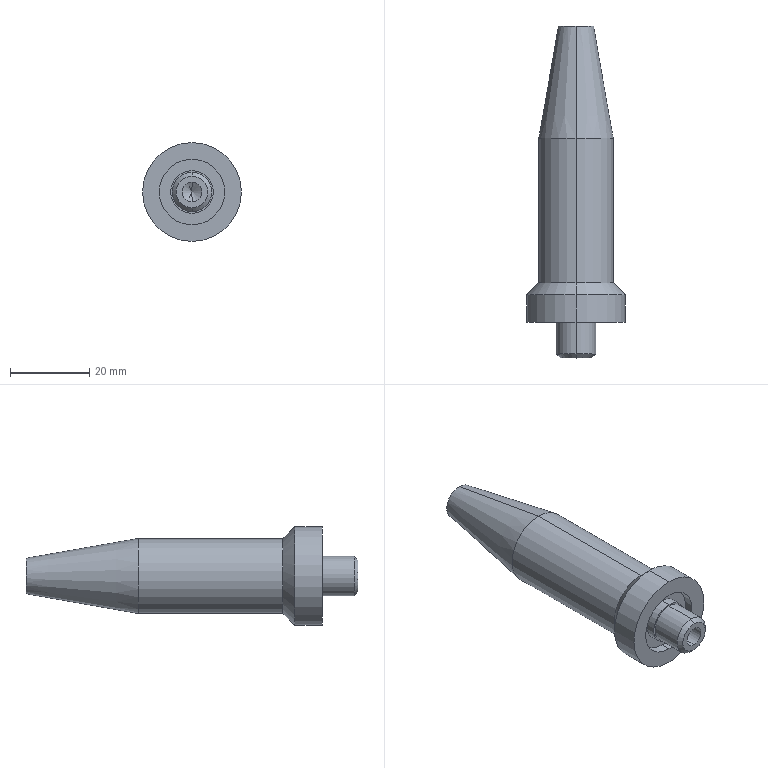Part | STEP file | PN_0062 | 1 solid | 25 faces | box 25 x 84 x 25 mm | volume 19612 mm3 | cylinder 12 | cone 8 | plane 5 | commonest cylinder face diameters 5 x2 10 x2 10.8 x2 16.6 x2 19 x2 25 x2
STEP:
#1=CARTESIAN_POINT('',(0.,0.,0.));
#2=DIRECTION('',(0.,0.,1.));
#3=DIRECTION('',(1.,0.,0.));
#4=AXIS2_PLACEMENT_3D('',#1,#2,#3);
#5=CARTESIAN_POINT('',(0.,75.,4.5));
#6=VERTEX_POINT('',#5);
#7=CARTESIAN_POINT('',(0.,75.,-4.5));
#8=VERTEX_POINT('',#7);
#9=CARTESIAN_POINT('',(0.,75.,0.));
#10=DIRECTION('',(0.,1.,0.));
#11=DIRECTION('',(0.,0.,1.));
#12=AXIS2_PLACEMENT_3D('',#9,#10,#11);
#13=CIRCLE('',#12,4.5);
#14=CARTESIAN_POINT('',(0.,75.,0.));
#15=DIRECTION('',(0.,-1.,0.));
#16=DIRECTION('',(0.,0.,-1.));
#17=AXIS2_PLACEMENT_3D('',#14,#15,#16);
#18=CONICAL_SURFACE('',#17,4.5,0.1745);
#19=CARTESIAN_POINT('',(3.142,0.));
#20=DIRECTION('',(-1.,0.));
#21=VECTOR('',#20,1.);
#22=LINE('',#19,#21);
#23=(GEOMETRIC_REPRESENTATION_CONTEXT(2)PARAMETRIC_REPRESENTATION_CONTEXT()REPRESENTATION_CONTEXT('',''));
#24=DEFINITIONAL_REPRESENTATION('',(#22),#23);
#25=PCURVE('',#18,#24);
#26=CARTESIAN_POINT('',(0.,75.,0.));
#27=DIRECTION('',(0.,1.,0.));
#28=DIRECTION('',(0.,0.,1.));
#29=AXIS2_PLACEMENT_3D('',#26,#27,#28);
#30=PLANE('',#29);
#31=CARTESIAN_POINT('',(0.,0.));
#32=DIRECTION('',(1.,0.));
#33=AXIS2_PLACEMENT_2D('',#31,#32);
#34=CIRCLE('',#33,4.5);
#35=(GEOMETRIC_REPRESENTATION_CONTEXT(2)PARAMETRIC_REPRESENTATION_CONTEXT()REPRESENTATION_CONTEXT('',''));
#36=DEFINITIONAL_REPRESENTATION('',(#34),#35);
#37=PCURVE('',#30,#36);
#38=SURFACE_CURVE('',#13,(#25,#37),.PCURVE_S1.);
#39=EDGE_CURVE('',#6,#8,#38,.T.);
#40=ORIENTED_EDGE('',*,*,#39,.F.);
#41=CARTESIAN_POINT('',(0.,46.644,9.5));
#42=VERTEX_POINT('',#41);
#43=CARTESIAN_POINT('',(0.,75.,4.5));
#44=DIRECTION('',(0.,-0.9848,0.1736));
#45=VECTOR('',#44,1.);
#46=LINE('',#43,#45);
#47=CARTESIAN_POINT('',(3.142,0.));
#48=DIRECTION('',(0.,1.));
#49=VECTOR('',#48,1.);
#50=LINE('',#47,#49);
#51=(GEOMETRIC_REPRESENTATION_CONTEXT(2)PARAMETRIC_REPRESENTATION_CONTEXT()REPRESENTATION_CONTEXT('',''));
#52=DEFINITIONAL_REPRESENTATION('',(#50),#51);
#53=PCURVE('',#18,#52);
#54=CARTESIAN_POINT('',(0.,75.,0.));
#55=DIRECTION('',(0.,-1.,0.));
#56=DIRECTION('',(0.,0.,-1.));
#57=AXIS2_PLACEMENT_3D('',#54,#55,#56);
#58=CONICAL_SURFACE('',#57,4.5,0.1745);
#59=CARTESIAN_POINT('',(3.142,0.));
#60=DIRECTION('',(0.,1.));
#61=VECTOR('',#60,1.);
#62=LINE('',#59,#61);
#63=(GEOMETRIC_REPRESENTATION_CONTEXT(2)PARAMETRIC_REPRESENTATION_CONTEXT()REPRESENTATION_CONTEXT('',''));
#64=DEFINITIONAL_REPRESENTATION('',(#62),#63);
#65=PCURVE('',#58,#64);
#66=SURFACE_CURVE('',#46,(#53,#65),.PCURVE_S1.);
#67=EDGE_CURVE('',#6,#42,#66,.T.);
#68=ORIENTED_EDGE('',*,*,#67,.T.);
#69=CARTESIAN_POINT('',(0.,46.644,-9.5));
#70=VERTEX_POINT('',#69);
#71=CARTESIAN_POINT('',(0.,46.644,0.));
#72=DIRECTION('',(0.,-1.,0.));
#73=DIRECTION('',(0.,0.,1.));
#74=AXIS2_PLACEMENT_3D('',#71,#72,#73);
#75=CIRCLE('',#74,9.5);
#76=CARTESIAN_POINT('',(-3.142,28.356));
#77=DIRECTION('',(1.,0.));
#78=VECTOR('',#77,1.);
#79=LINE('',#76,#78);
#80=(GEOMETRIC_REPRESENTATION_CONTEXT(2)PARAMETRIC_REPRESENTATION_CONTEXT()REPRESENTATION_CONTEXT('',''));
#81=DEFINITIONAL_REPRESENTATION('',(#79),#80);
#82=PCURVE('',#18,#81);
#83=CARTESIAN_POINT('',(0.,75.,0.));
#84=DIRECTION('',(0.,-1.,0.));
#85=DIRECTION('',(0.,0.,-1.));
#86=AXIS2_PLACEMENT_3D('',#83,#84,#85);
#87=CYLINDRICAL_SURFACE('',#86,9.5);
#88=CARTESIAN_POINT('',(-3.142,28.356));
#89=DIRECTION('',(1.,0.));
#90=VECTOR('',#89,1.);
#91=LINE('',#88,#90);
#92=(GEOMETRIC_REPRESENTATION_CONTEXT(2)PARAMETRIC_REPRESENTATION_CONTEXT()REPRESENTATION_CONTEXT('',''));
#93=DEFINITIONAL_REPRESENTATION('',(#91),#92);
#94=PCURVE('',#87,#93);
#95=SURFACE_CURVE('',#75,(#82,#94),.PCURVE_S1.);
#96=EDGE_CURVE('',#70,#42,#95,.T.);
#97=ORIENTED_EDGE('',*,*,#96,.F.);
#98=CARTESIAN_POINT('',(0.,75.,-4.5));
#99=DIRECTION('',(0.,-0.9848,-0.1736));
#100=VECTOR('',#99,1.);
#101=LINE('',#98,#100);
#102=CARTESIAN_POINT('',(0.,0.));
#103=DIRECTION('',(0.,1.));
#104=VECTOR('',#103,1.);
#105=LINE('',#102,#104);
#106=(GEOMETRIC_REPRESENTATION_CONTEXT(2)PARAMETRIC_REPRESENTATION_CONTEXT()REPRESENTATION_CONTEXT('',''));
#107=DEFINITIONAL_REPRESENTATION('',(#105),#106);
#108=PCURVE('',#18,#107);
#109=CARTESIAN_POINT('',(6.283,0.));
#110=DIRECTION('',(0.,1.));
#111=VECTOR('',#110,1.);
#112=LINE('',#109,#111);
#113=(GEOMETRIC_REPRESENTATION_CONTEXT(2)PARAMETRIC_REPRESENTATION_CONTEXT()REPRESENTATION_CONTEXT('',''));
#114=DEFINITIONAL_REPRESENTATION('',(#112),#113);
#115=PCURVE('',#58,#114);
#116=SURFACE_CURVE('',#101,(#108,#115),.PCURVE_S1.);
#117=EDGE_CURVE('',#8,#70,#116,.T.);
#118=ORIENTED_EDGE('',*,*,#117,.F.);
#119=EDGE_LOOP('',(#40,#68,#97,#118));
#120=FACE_BOUND('',#119,.T.);
#121=ADVANCED_FACE('',(#120),#18,.T.);
#122=CARTESIAN_POINT('',(0.,6.,-2.5));
#123=VERTEX_POINT('',#122);
#124=CARTESIAN_POINT('',(0.,-9.,-2.5));
#125=VERTEX_POINT('',#124);
#126=CARTESIAN_POINT('',(0.,-9.,-2.5));
#127=DIRECTION('',(0.,-1.,0.));
#128=VECTOR('',#127,1.);
#129=LINE('',#126,#128);
#130=CARTESIAN_POINT('',(0.,-9.,0.));
#131=DIRECTION('',(0.,-1.,0.));
#132=DIRECTION('',(0.,0.,-1.));
#133=AXIS2_PLACEMENT_3D('',#130,#131,#132);
#134=CYLINDRICAL_SURFACE('',#133,2.5);
#135=CARTESIAN_POINT('',(6.283,0.));
#136=DIRECTION('',(0.,1.));
#137=VECTOR('',#136,1.);
#138=LINE('',#135,#137);
#139=(GEOMETRIC_REPRESENTATION_CONTEXT(2)PARAMETRIC_REPRESENTATION_CONTEXT()REPRESENTATION_CONTEXT('',''));
#140=DEFINITIONAL_REPRESENTATION('',(#138),#139);
#141=PCURVE('',#134,#140);
#142=CARTESIAN_POINT('',(0.,-9.,0.));
#143=DIRECTION('',(0.,-1.,0.));
#144=DIRECTION('',(0.,0.,-1.));
#145=AXIS2_PLACEMENT_3D('',#142,#143,#144);
#146=CYLINDRICAL_SURFACE('',#145,2.5);
#147=CARTESIAN_POINT('',(0.,0.));
#148=DIRECTION('',(0.,1.));
#149=VECTOR('',#148,1.);
#150=LINE('',#147,#149);
#151=(GEOMETRIC_REPRESENTATION_CONTEXT(2)PARAMETRIC_REPRESENTATION_CONTEXT()REPRESENTATION_CONTEXT('',''));
#152=DEFINITIONAL_REPRESENTATION('',(#150),#151);
#153=PCURVE('',#146,#152);
#154=SURFACE_CURVE('',#129,(#141,#153),.PCURVE_S1.);
#155=EDGE_CURVE('',#123,#125,#154,.T.);
#156=ORIENTED_EDGE('',*,*,#155,.T.);
#157=CARTESIAN_POINT('',(0.,-9.,2.5));
#158=VERTEX_POINT('',#157);
#159=CARTESIAN_POINT('',(0.,-9.,0.));
#160=DIRECTION('',(0.,-1.,0.));
#161=DIRECTION('',(0.,0.,-1.));
#162=AXIS2_PLACEMENT_3D('',#159,#160,#161);
#163=CIRCLE('',#162,2.5);
#164=CARTESIAN_POINT('',(0.,0.));
#165=DIRECTION('',(1.,0.));
#166=VECTOR('',#165,1.);
#167=LINE('',#164,#166);
#168=(GEOMETRIC_REPRESENTATION_CONTEXT(2)PARAMETRIC_REPRESENTATION_CONTEXT()REPRESENTATION_CONTEXT('',''));
#169=DEFINITIONAL_REPRESENTATION('',(#167),#168);
#170=PCURVE('',#134,#169);
#171=CARTESIAN_POINT('',(0.,-9.,0.));
#172=DIRECTION('',(0.,-1.,0.));
#173=DIRECTION('',(0.,0.,-1.));
#174=AXIS2_PLACEMENT_3D('',#171,#172,#173);
#175=PLANE('',#174);
#176=CARTESIAN_POINT('',(0.,0.));
#177=DIRECTION('',(1.,0.));
#178=AXIS2_PLACEMENT_2D('',#176,#177);
#179=CIRCLE('',#178,2.5);
#180=(GEOMETRIC_REPRESENTATION_CONTEXT(2)PARAMETRIC_REPRESENTATION_CONTEXT()REPRESENTATION_CONTEXT('',''));
#181=DEFINITIONAL_REPRESENTATION('',(#179),#180);
#182=PCURVE('',#175,#181);
#183=SURFACE_CURVE('',#163,(#170,#182),.PCURVE_S1.);
#184=EDGE_CURVE('',#158,#125,#183,.T.);
#185=ORIENTED_EDGE('',*,*,#184,.F.);
#186=CARTESIAN_POINT('',(0.,6.,2.5));
#187=VERTEX_POINT('',#186);
#188=CARTESIAN_POINT('',(0.,-9.,2.5));
#189=DIRECTION('',(0.,-1.,0.));
#190=VECTOR('',#189,1.);
#191=LINE('',#188,#190);
#192=CARTESIAN_POINT('',(3.142,0.));
#193=DIRECTION('',(0.,1.));
#194=VECTOR('',#193,1.);
#195=LINE('',#192,#194);
#196=(GEOMETRIC_REPRESENTATION_CONTEXT(2)PARAMETRIC_REPRESENTATION_CONTEXT()REPRESENTATION_CONTEXT('',''));
#197=DEFINITIONAL_REPRESENTATION('',(#195),#196);
#198=PCURVE('',#134,#197);
#199=CARTESIAN_POINT('',(3.142,0.));
#200=DIRECTION('',(0.,1.));
#201=VECTOR('',#200,1.);
#202=LINE('',#199,#201);
#203=(GEOMETRIC_REPRESENTATION_CONTEXT(2)PARAMETRIC_REPRESENTATION_CONTEXT()REPRESENTATION_CONTEXT('',''));
#204=DEFINITIONAL_REPRESENTATION('',(#202),#203);
#205=PCURVE('',#146,#204);
#206=SURFACE_CURVE('',#191,(#198,#205),.PCURVE_S1.);
#207=EDGE_CURVE('',#187,#158,#206,.T.);
#208=ORIENTED_EDGE('',*,*,#207,.F.);
#209=CARTESIAN_POINT('',(0.,6.,0.));
#210=DIRECTION('',(0.,-1.,0.));
#211=DIRECTION('',(0.,0.,-1.));
#212=AXIS2_PLACEMENT_3D('',#209,#210,#211);
#213=CIRCLE('',#212,2.5);
#214=CARTESIAN_POINT('',(0.,-15.));
#215=DIRECTION('',(1.,0.));
#216=VECTOR('',#215,1.);
#217=LINE('',#214,#216);
#218=(GEOMETRIC_REPRESENTATION_CONTEXT(2)PARAMETRIC_REPRESENTATION_CONTEXT()REPRESENTATION_CONTEXT('',''));
#219=DEFINITIONAL_REPRESENTATION('',(#217),#218);
#220=PCURVE('',#134,#219);
#221=CARTESIAN_POINT('',(0.,6.,0.));
#222=DIRECTION('',(0.,-1.,0.));
#223=DIRECTION('',(0.,0.,-1.));
#224=AXIS2_PLACEMENT_3D('',#221,#222,#223);
#225=CONICAL_SURFACE('',#224,2.5,1.03);
#226=CARTESIAN_POINT('',(0.,0.));
#227=DIRECTION('',(1.,0.));
#228=VECTOR('',#227,1.);
#229=LINE('',#226,#228);
#230=(GEOMETRIC_REPRESENTATION_CONTEXT(2)PARAMETRIC_REPRESENTATION_CONTEXT()REPRESENTATION_CONTEXT('',''));
#231=DEFINITIONAL_REPRESENTATION('',(#229),#230);
#232=PCURVE('',#225,#231);
#233=SURFACE_CURVE('',#213,(#220,#232),.PCURVE_S1.);
#234=EDGE_CURVE('',#187,#123,#233,.T.);
#235=ORIENTED_EDGE('',*,*,#234,.T.);
#236=EDGE_LOOP('',(#156,#185,#208,#235));
#237=FACE_BOUND('',#236,.F.);
#238=ADVANCED_FACE('',(#237),#134,.F.);
#239=ORIENTED_EDGE('',*,*,#234,.F.);
#240=CARTESIAN_POINT('',(0.,7.502,0.));
#241=VERTEX_POINT('',#240);
#242=CARTESIAN_POINT('',(0.,6.,2.5));
#243=DIRECTION('',(0.,-0.515,0.8572));
#244=VECTOR('',#243,1.);
#245=LINE('',#242,#244);
#246=CARTESIAN_POINT('',(3.142,0.));
#247=DIRECTION('',(0.,1.));
#248=VECTOR('',#247,1.);
#249=LINE('',#246,#248);
#250=(GEOMETRIC_REPRESENTATION_CONTEXT(2)PARAMETRIC_REPRESENTATION_CONTEXT()REPRESENTATION_CONTEXT('',''));
#251=DEFINITIONAL_REPRESENTATION('',(#249),#250);
#252=PCURVE('',#225,#251);
#253=CARTESIAN_POINT('',(0.,6.,0.));
#254=DIRECTION('',(0.,-1.,0.));
#255=DIRECTION('',(0.,0.,-1.));
#256=AXIS2_PLACEMENT_3D('',#253,#254,#255);
#257=CONICAL_SURFACE('',#256,2.5,1.03);
#258=CARTESIAN_POINT('',(3.142,0.));
#259=DIRECTION('',(0.,1.));
#260=VECTOR('',#259,1.);
#261=LINE('',#258,#260);
#262=(GEOMETRIC_REPRESENTATION_CONTEXT(2)PARAMETRIC_REPRESENTATION_CONTEXT()REPRESENTATION_CONTEXT('',''));
#263=DEFINITIONAL_REPRESENTATION('',(#261),#262);
#264=PCURVE('',#257,#263);
#265=SURFACE_CURVE('',#245,(#252,#264),.PCURVE_S1.);
#266=EDGE_CURVE('',#241,#187,#265,.T.);
#267=ORIENTED_EDGE('',*,*,#266,.F.);
#268=CARTESIAN_POINT('',(0.,6.,-2.5));
#269=DIRECTION('',(0.,-0.515,-0.8572));
#270=VECTOR('',#269,1.);
#271=LINE('',#268,#270);
#272=CARTESIAN_POINT('',(6.283,0.));
#273=DIRECTION('',(0.,1.));
#274=VECTOR('',#273,1.);
#275=LINE('',#272,#274);
#276=(GEOMETRIC_REPRESENTATION_CONTEXT(2)PARAMETRIC_REPRESENTATION_CONTEXT()REPRESENTATION_CONTEXT('',''));
#277=DEFINITIONAL_REPRESENTATION('',(#275),#276);
#278=PCURVE('',#225,#277);
#279=CARTESIAN_POINT('',(0.,0.));
#280=DIRECTION('',(0.,1.));
#281=VECTOR('',#280,1.);
#282=LINE('',#279,#281);
#283=(GEOMETRIC_REPRESENTATION_CONTEXT(2)PARAMETRIC_REPRESENTATION_CONTEXT()REPRESENTATION_CONTEXT('',''));
#284=DEFINITIONAL_REPRESENTATION('',(#282),#283);
#285=PCURVE('',#257,#284);
#286=SURFACE_CURVE('',#271,(#278,#285),.PCURVE_S1.);
#287=EDGE_CURVE('',#241,#123,#286,.T.);
#288=ORIENTED_EDGE('',*,*,#287,.T.);
#289=EDGE_LOOP('',(#239,#267,#288));
#290=FACE_BOUND('',#289,.F.);
#291=ADVANCED_FACE('',(#290),#225,.F.);
#292=CARTESIAN_POINT('',(0.,10.,-9.5));
#293=VERTEX_POINT('',#292);
#294=CARTESIAN_POINT('',(0.,10.,9.5));
#295=VERTEX_POINT('',#294);
#296=CARTESIAN_POINT('',(0.,10.,0.));
#297=DIRECTION('',(0.,-1.,0.));
#298=DIRECTION('',(0.,0.,-1.));
#299=AXIS2_PLACEMENT_3D('',#296,#297,#298);
#300=CIRCLE('',#299,9.5);
#301=CARTESIAN_POINT('',(0.,7.,0.));
#302=DIRECTION('',(0.,-1.,0.));
#303=DIRECTION('',(0.,0.,-1.));
#304=AXIS2_PLACEMENT_3D('',#301,#302,#303);
#305=CONICAL_SURFACE('',#304,12.5,0.7854);
#306=CARTESIAN_POINT('',(0.,-3.));
#307=DIRECTION('',(1.,0.));
#308=VECTOR('',#307,1.);
#309=LINE('',#306,#308);
#310=(GEOMETRIC_REPRESENTATION_CONTEXT(2)PARAMETRIC_REPRESENTATION_CONTEXT()REPRESENTATION_CONTEXT('',''));
#311=DEFINITIONAL_REPRESENTATION('',(#309),#310);
#312=PCURVE('',#305,#311);
#313=CARTESIAN_POINT('',(0.,65.));
#314=DIRECTION('',(1.,0.));
#315=VECTOR('',#314,1.);
#316=LINE('',#313,#315);
#317=(GEOMETRIC_REPRESENTATION_CONTEXT(2)PARAMETRIC_REPRESENTATION_CONTEXT()REPRESENTATION_CONTEXT('',''));
#318=DEFINITIONAL_REPRESENTATION('',(#316),#317);
#319=PCURVE('',#87,#318);
#320=SURFACE_CURVE('',#300,(#312,#319),.PCURVE_S1.);
#321=EDGE_CURVE('',#293,#295,#320,.T.);
#322=ORIENTED_EDGE('',*,*,#321,.T.);
#323=CARTESIAN_POINT('',(0.,7.,12.5));
#324=VERTEX_POINT('',#323);
#325=CARTESIAN_POINT('',(0.,7.,12.5));
#326=DIRECTION('',(0.,-0.7071,0.7071));
#327=VECTOR('',#326,1.);
#328=LINE('',#325,#327);
#329=CARTESIAN_POINT('',(3.142,0.));
#330=DIRECTION('',(0.,1.));
#331=VECTOR('',#330,1.);
#332=LINE('',#329,#331);
#333=(GEOMETRIC_REPRESENTATION_CONTEXT(2)PARAMETRIC_REPRESENTATION_CONTEXT()REPRESENTATION_CONTEXT('',''));
#334=DEFINITIONAL_REPRESENTATION('',(#332),#333);
#335=PCURVE('',#305,#334);
#336=CARTESIAN_POINT('',(0.,7.,0.));
#337=DIRECTION('',(0.,-1.,0.));
#338=DIRECTION('',(0.,0.,-1.));
#339=AXIS2_PLACEMENT_3D('',#336,#337,#338);
#340=CONICAL_SURFACE('',#339,12.5,0.7854);
#341=CARTESIAN_POINT('',(3.142,0.));
#342=DIRECTION('',(0.,1.));
#343=VECTOR('',#342,1.);
#344=LINE('',#341,#343);
#345=(GEOMETRIC_REPRESENTATION_CONTEXT(2)PARAMETRIC_REPRESENTATION_CONTEXT()REPRESENTATION_CONTEXT('',''));
#346=DEFINITIONAL_REPRESENTATION('',(#344),#345);
#347=PCURVE('',#340,#346);
#348=SURFACE_CURVE('',#328,(#335,#347),.PCURVE_S1.);
#349=EDGE_CURVE('',#295,#324,#348,.T.);
#350=ORIENTED_EDGE('',*,*,#349,.T.);
#351=CARTESIAN_POINT('',(0.,7.,-12.5));
#352=VERTEX_POINT('',#351);
#353=CARTESIAN_POINT('',(0.,7.,0.));
#354=DIRECTION('',(0.,-1.,0.));
#355=DIRECTION('',(0.,0.,-1.));
#356=AXIS2_PLACEMENT_3D('',#353,#354,#355);
#357=CIRCLE('',#356,12.5);
#358=CARTESIAN_POINT('',(0.,0.));
#359=DIRECTION('',(1.,0.));
#360=VECTOR('',#359,1.);
#361=LINE('',#358,#360);
#362=(GEOMETRIC_REPRESENTATION_CONTEXT(2)PARAMETRIC_REPRESENTATION_CONTEXT()REPRESENTATION_CONTEXT('',''));
#363=DEFINITIONAL_REPRESENTATION('',(#361),#362);
#364=PCURVE('',#305,#363);
#365=CARTESIAN_POINT('',(0.,10.,0.));
#366=DIRECTION('',(0.,-1.,0.));
#367=DIRECTION('',(0.,0.,-1.));
#368=AXIS2_PLACEMENT_3D('',#365,#366,#367);
#369=CYLINDRICAL_SURFACE('',#368,12.5);
#370=CARTESIAN_POINT('',(0.,3.));
#371=DIRECTION('',(1.,0.));
#372=VECTOR('',#371,1.);
#373=LINE('',#370,#372);
#374=(GEOMETRIC_REPRESENTATION_CONTEXT(2)PARAMETRIC_REPRESENTATION_CONTEXT()REPRESENTATION_CONTEXT('',''));
#375=DEFINITIONAL_REPRESENTATION('',(#373),#374);
#376=PCURVE('',#369,#375);
#377=SURFACE_CURVE('',#357,(#364,#376),.PCURVE_S1.);
#378=EDGE_CURVE('',#352,#324,#377,.T.);
#379=ORIENTED_EDGE('',*,*,#378,.F.);
#380=CARTESIAN_POINT('',(0.,7.,-12.5));
#381=DIRECTION('',(0.,-0.7071,-0.7071));
#382=VECTOR('',#381,1.);
#383=LINE('',#380,#382);
#384=CARTESIAN_POINT('',(0.,0.));
#385=DIRECTION('',(0.,1.));
#386=VECTOR('',#385,1.);
#387=LINE('',#384,#386);
#388=(GEOMETRIC_REPRESENTATION_CONTEXT(2)PARAMETRIC_REPRESENTATION_CONTEXT()REPRESENTATION_CONTEXT('',''));
#389=DEFINITIONAL_REPRESENTATION('',(#387),#388);
#390=PCURVE('',#305,#389);
#391=CARTESIAN_POINT('',(6.283,0.));
#392=DIRECTION('',(0.,1.));
#393=VECTOR('',#392,1.);
#394=LINE('',#391,#393);
#395=(GEOMETRIC_REPRESENTATION_CONTEXT(2)PARAMETRIC_REPRESENTATION_CONTEXT()REPRESENTATION_CONTEXT('',''));
#396=DEFINITIONAL_REPRESENTATION('',(#394),#395);
#397=PCURVE('',#340,#396);
#398=SURFACE_CURVE('',#383,(#390,#397),.PCURVE_S1.);
#399=EDGE_CURVE('',#293,#352,#398,.T.);
#400=ORIENTED_EDGE('',*,*,#399,.F.);
#401=EDGE_LOOP('',(#322,#350,#379,#400));
#402=FACE_BOUND('',#401,.T.);
#403=ADVANCED_FACE('',(#402),#305,.T.);
#404=ORIENTED_EDGE('',*,*,#96,.T.);
#405=CARTESIAN_POINT('',(0.,75.,9.5));
#406=DIRECTION('',(0.,-1.,0.));
#407=VECTOR('',#406,1.);
#408=LINE('',#405,#407);
#409=CARTESIAN_POINT('',(3.142,0.));
#410=DIRECTION('',(0.,1.));
#411=VECTOR('',#410,1.);
#412=LINE('',#409,#411);
#413=(GEOMETRIC_REPRESENTATION_CONTEXT(2)PARAMETRIC_REPRESENTATION_CONTEXT()REPRESENTATION_CONTEXT('',''));
#414=DEFINITIONAL_REPRESENTATION('',(#412),#413);
#415=PCURVE('',#87,#414);
#416=CARTESIAN_POINT('',(0.,75.,0.));
#417=DIRECTION('',(0.,-1.,0.));
#418=DIRECTION('',(0.,0.,-1.));
#419=AXIS2_PLACEMENT_3D('',#416,#417,#418);
#420=CYLINDRICAL_SURFACE('',#419,9.5);
#421=CARTESIAN_POINT('',(3.142,0.));
#422=DIRECTION('',(0.,1.));
#423=VECTOR('',#422,1.);
#424=LINE('',#421,#423);
#425=(GEOMETRIC_REPRESENTATION_CONTEXT(2)PARAMETRIC_REPRESENTATION_CONTEXT()REPRESENTATION_CONTEXT('',''));
#426=DEFINITIONAL_REPRESENTATION('',(#424),#425);
#427=PCURVE('',#420,#426);
#428=SURFACE_CURVE('',#408,(#415,#427),.PCURVE_S1.);
#429=EDGE_CURVE('',#42,#295,#428,.T.);
#430=ORIENTED_EDGE('',*,*,#429,.T.);
#431=ORIENTED_EDGE('',*,*,#321,.F.);
#432=CARTESIAN_POINT('',(0.,75.,-9.5));
#433=DIRECTION('',(0.,-1.,0.));
#434=VECTOR('',#433,1.);
#435=LINE('',#432,#434);
#436=CARTESIAN_POINT('',(0.,0.));
#437=DIRECTION('',(0.,1.));
#438=VECTOR('',#437,1.);
#439=LINE('',#436,#438);
#440=(GEOMETRIC_REPRESENTATION_CONTEXT(2)PARAMETRIC_REPRESENTATION_CONTEXT()REPRESENTATION_CONTEXT('',''));
#441=DEFINITIONAL_REPRESENTATION('',(#439),#440);
#442=PCURVE('',#87,#441);
#443=CARTESIAN_POINT('',(6.283,0.));
#444=DIRECTION('',(0.,1.));
#445=VECTOR('',#444,1.);
#446=LINE('',#443,#445);
#447=(GEOMETRIC_REPRESENTATION_CONTEXT(2)PARAMETRIC_REPRESENTATION_CONTEXT()REPRESENTATION_CONTEXT('',''));
#448=DEFINITIONAL_REPRESENTATION('',(#446),#447);
#449=PCURVE('',#420,#448);
#450=SURFACE_CURVE('',#435,(#442,#449),.PCURVE_S1.);
#451=EDGE_CURVE('',#70,#293,#450,.T.);
#452=ORIENTED_EDGE('',*,*,#451,.F.);
#453=EDGE_LOOP('',(#404,#430,#431,#452));
#454=FACE_BOUND('',#453,.T.);
#455=ADVANCED_FACE('',(#454),#87,.T.);
#456=ORIENTED_EDGE('',*,*,#378,.T.);
#457=CARTESIAN_POINT('',(0.,0.,12.5));
#458=VERTEX_POINT('',#457);
#459=CARTESIAN_POINT('',(0.,10.,12.5));
#460=DIRECTION('',(0.,-1.,0.));
#461=VECTOR('',#460,1.);
#462=LINE('',#459,#461);
#463=CARTESIAN_POINT('',(3.142,0.));
#464=DIRECTION('',(0.,1.));
#465=VECTOR('',#464,1.);
#466=LINE('',#463,#465);
#467=(GEOMETRIC_REPRESENTATION_CONTEXT(2)PARAMETRIC_REPRESENTATION_CONTEXT()REPRESENTATION_CONTEXT('',''));
#468=DEFINITIONAL_REPRESENTATION('',(#466),#467);
#469=PCURVE('',#369,#468);
#470=CARTESIAN_POINT('',(0.,10.,0.));
#471=DIRECTION('',(0.,-1.,0.));
#472=DIRECTION('',(0.,0.,-1.));
#473=AXIS2_PLACEMENT_3D('',#470,#471,#472);
#474=CYLINDRICAL_SURFACE('',#473,12.5);
#475=CARTESIAN_POINT('',(3.142,0.));
#476=DIRECTION('',(0.,1.));
#477=VECTOR('',#476,1.);
#478=LINE('',#475,#477);
#479=(GEOMETRIC_REPRESENTATION_CONTEXT(2)PARAMETRIC_REPRESENTATION_CONTEXT()REPRESENTATION_CONTEXT('',''));
#480=DEFINITIONAL_REPRESENTATION('',(#478),#479);
#481=PCURVE('',#474,#480);
#482=SURFACE_CURVE('',#462,(#469,#481),.PCURVE_S1.);
#483=EDGE_CURVE('',#324,#458,#482,.T.);
#484=ORIENTED_EDGE('',*,*,#483,.T.);
#485=CARTESIAN_POINT('',(0.,0.,-12.5));
#486=VERTEX_POINT('',#485);
#487=CARTESIAN_POINT('',(0.,0.,0.));
#488=DIRECTION('',(0.,-1.,0.));
#489=DIRECTION('',(0.,0.,-1.));
#490=AXIS2_PLACEMENT_3D('',#487,#488,#489);
#491=CIRCLE('',#490,12.5);
#492=CARTESIAN_POINT('',(0.,10.));
#493=DIRECTION('',(1.,0.));
#494=VECTOR('',#493,1.);
#495=LINE('',#492,#494);
#496=(GEOMETRIC_REPRESENTATION_CONTEXT(2)PARAMETRIC_REPRESENTATION_CONTEXT()REPRESENTATION_CONTEXT('',''));
#497=DEFINITIONAL_REPRESENTATION('',(#495),#496);
#498=PCURVE('',#369,#497);
#499=CARTESIAN_POINT('',(0.,0.,0.));
#500=DIRECTION('',(0.,1.,0.));
#501=DIRECTION('',(0.,0.,1.));
#502=AXIS2_PLACEMENT_3D('',#499,#500,#501);
#503=PLANE('',#502);
#504=CARTESIAN_POINT('',(-12.5,0.));
#505=CARTESIAN_POINT('',(-12.5,21.651));
#506=CARTESIAN_POINT('',(6.25,10.825));
#507=CARTESIAN_POINT('',(25.,0.));
#508=CARTESIAN_POINT('',(6.25,-10.825));
#509=CARTESIAN_POINT('',(-12.5,-21.651));
#510=CARTESIAN_POINT('',(-12.5,0.));
#511=(BOUNDED_CURVE()B_SPLINE_CURVE(2,(#504,#505,#506,#507,#508,#509,#510),.UNSPECIFIED.,.T.,.F.)B_SPLINE_CURVE_WITH_KNOTS((1,2,2,2,2,1),(-2.094,0.,2.094,4.189,6.283,8.378),.UNSPECIFIED.)CURVE()GEOMETRIC_REPRESENTATION_ITEM()RATIONAL_B_SPLINE_CURVE((1.,0.5,1.,0.5,1.,0.5,1.))REPRESENTATION_ITEM(''));
#512=(GEOMETRIC_REPRESENTATION_CONTEXT(2)PARAMETRIC_REPRESENTATION_CONTEXT()REPRESENTATION_CONTEXT('',''));
#513=DEFINITIONAL_REPRESENTATION('',(#511),#512);
#514=PCURVE('',#503,#513);
#515=SURFACE_CURVE('',#491,(#498,#514),.PCURVE_S1.);
#516=EDGE_CURVE('',#486,#458,#515,.T.);
#517=ORIENTED_EDGE('',*,*,#516,.F.);
#518=CARTESIAN_POINT('',(0.,10.,-12.5));
#519=DIRECTION('',(0.,-1.,0.));
#520=VECTOR('',#519,1.);
#521=LINE('',#518,#520);
#522=CARTESIAN_POINT('',(0.,0.));
#523=DIRECTION('',(0.,1.));
#524=VECTOR('',#523,1.);
#525=LINE('',#522,#524);
#526=(GEOMETRIC_REPRESENTATION_CONTEXT(2)PARAMETRIC_REPRESENTATION_CONTEXT()REPRESENTATION_CONTEXT('',''));
#527=DEFINITIONAL_REPRESENTATION('',(#525),#526);
#528=PCURVE('',#369,#527);
#529=CARTESIAN_POINT('',(6.283,0.));
#530=DIRECTION('',(0.,1.));
#531=VECTOR('',#530,1.);
#532=LINE('',#529,#531);
#533=(GEOMETRIC_REPRESENTATION_CONTEXT(2)PARAMETRIC_REPRESENTATION_CONTEXT()REPRESENTATION_CONTEXT('',''));
#534=DEFINITIONAL_REPRESENTATION('',(#532),#533);
#535=PCURVE('',#474,#534);
#536=SURFACE_CURVE('',#521,(#528,#535),.PCURVE_S1.);
#537=EDGE_CURVE('',#352,#486,#536,.T.);
#538=ORIENTED_EDGE('',*,*,#537,.F.);
#539=EDGE_LOOP('',(#456,#484,#517,#538));
#540=FACE_BOUND('',#539,.T.);
#541=ADVANCED_FACE('',(#540),#369,.T.);
#542=CARTESIAN_POINT('',(0.,2.4,-5.4));
#543=VERTEX_POINT('',#542);
#544=CARTESIAN_POINT('',(0.,2.4,5.4));
#545=VERTEX_POINT('',#544);
#546=CARTESIAN_POINT('',(0.,2.4,0.));
#547=DIRECTION('',(0.,-1.,0.));
#548=DIRECTION('',(0.,0.,-1.));
#549=AXIS2_PLACEMENT_3D('',#546,#547,#548);
#550=CIRCLE('',#549,5.4);
#551=CARTESIAN_POINT('',(0.,2.4,0.));
#552=DIRECTION('',(0.,-1.,0.));
#553=DIRECTION('',(0.,0.,-1.));
#554=AXIS2_PLACEMENT_3D('',#551,#552,#553);
#555=CYLINDRICAL_SURFACE('',#554,5.4);
#556=CARTESIAN_POINT('',(0.,0.));
#557=DIRECTION('',(1.,0.));
#558=VECTOR('',#557,1.);
#559=LINE('',#556,#558);
#560=(GEOMETRIC_REPRESENTATION_CONTEXT(2)PARAMETRIC_REPRESENTATION_CONTEXT()REPRESENTATION_CONTEXT('',''));
#561=DEFINITIONAL_REPRESENTATION('',(#559),#560);
#562=PCURVE('',#555,#561);
#563=CARTESIAN_POINT('',(0.,2.4,0.));
#564=DIRECTION('',(0.,-1.,0.));
#565=DIRECTION('',(0.,0.,-1.));
#566=AXIS2_PLACEMENT_3D('',#563,#564,#565);
#567=PLANE('',#566);
#568=CARTESIAN_POINT('',(0.,0.));
#569=DIRECTION('',(1.,0.));
#570=AXIS2_PLACEMENT_2D('',#568,#569);
#571=CIRCLE('',#570,5.4);
#572=(GEOMETRIC_REPRESENTATION_CONTEXT(2)PARAMETRIC_REPRESENTATION_CONTEXT()REPRESENTATION_CONTEXT('',''));
#573=DEFINITIONAL_REPRESENTATION('',(#571),#572);
#574=PCURVE('',#567,#573);
#575=SURFACE_CURVE('',#550,(#562,#574),.PCURVE_S1.);
#576=EDGE_CURVE('',#543,#545,#575,.T.);
#577=ORIENTED_EDGE('',*,*,#576,.T.);
#578=CARTESIAN_POINT('',(0.,0.,5.4));
#579=VERTEX_POINT('',#578);
#580=CARTESIAN_POINT('',(0.,2.4,5.4));
#581=DIRECTION('',(0.,-1.,0.));
#582=VECTOR('',#581,1.);
#583=LINE('',#580,#582);
#584=CARTESIAN_POINT('',(3.142,0.));
#585=DIRECTION('',(0.,1.));
#586=VECTOR('',#585,1.);
#587=LINE('',#584,#586);
#588=(GEOMETRIC_REPRESENTATION_CONTEXT(2)PARAMETRIC_REPRESENTATION_CONTEXT()REPRESENTATION_CONTEXT('',''));
#589=DEFINITIONAL_REPRESENTATION('',(#587),#588);
#590=PCURVE('',#555,#589);
#591=CARTESIAN_POINT('',(0.,2.4,0.));
#592=DIRECTION('',(0.,-1.,0.));
#593=DIRECTION('',(0.,0.,-1.));
#594=AXIS2_PLACEMENT_3D('',#591,#592,#593);
#595=CYLINDRICAL_SURFACE('',#594,5.4);
#596=CARTESIAN_POINT('',(3.142,0.));
#597=DIRECTION('',(0.,1.));
#598=VECTOR('',#597,1.);
#599=LINE('',#596,#598);
#600=(GEOMETRIC_REPRESENTATION_CONTEXT(2)PARAMETRIC_REPRESENTATION_CONTEXT()REPRESENTATION_CONTEXT('',''));
#601=DEFINITIONAL_REPRESENTATION('',(#599),#600);
#602=PCURVE('',#595,#601);
#603=SURFACE_CURVE('',#583,(#590,#602),.PCURVE_S1.);
#604=EDGE_CURVE('',#545,#579,#603,.T.);
#605=ORIENTED_EDGE('',*,*,#604,.T.);
#606=CARTESIAN_POINT('',(0.,0.,-5.4));
#607=VERTEX_POINT('',#606);
#608=CARTESIAN_POINT('',(0.,0.,0.));
#609=DIRECTION('',(0.,-1.,0.));
#610=DIRECTION('',(0.,0.,-1.));
#611=AXIS2_PLACEMENT_3D('',#608,#609,#610);
#612=CIRCLE('',#611,5.4);
#613=CARTESIAN_POINT('',(0.,2.4));
#614=DIRECTION('',(1.,0.));
#615=VECTOR('',#614,1.);
#616=LINE('',#613,#615);
#617=(GEOMETRIC_REPRESENTATION_CONTEXT(2)PARAMETRIC_REPRESENTATION_CONTEXT()REPRESENTATION_CONTEXT('',''));
#618=DEFINITIONAL_REPRESENTATION('',(#616),#617);
#619=PCURVE('',#555,#618);
#620=CARTESIAN_POINT('',(0.,0.,0.));
#621=DIRECTION('',(0.,1.,0.));
#622=DIRECTION('',(0.,0.,1.));
#623=AXIS2_PLACEMENT_3D('',#620,#621,#622);
#624=PLANE('',#623);
#625=CARTESIAN_POINT('',(-5.4,0.));
#626=CARTESIAN_POINT('',(-5.4,9.353));
#627=CARTESIAN_POINT('',(2.7,4.677));
#628=CARTESIAN_POINT('',(10.8,0.));
#629=CARTESIAN_POINT('',(2.7,-4.677));
#630=CARTESIAN_POINT('',(-5.4,-9.353));
#631=CARTESIAN_POINT('',(-5.4,0.));
#632=(BOUNDED_CURVE()B_SPLINE_CURVE(2,(#625,#626,#627,#628,#629,#630,#631),.UNSPECIFIED.,.T.,.F.)B_SPLINE_CURVE_WITH_KNOTS((1,2,2,2,2,1),(-2.094,0.,2.094,4.189,6.283,8.378),.UNSPECIFIED.)CURVE()GEOMETRIC_REPRESENTATION_ITEM()RATIONAL_B_SPLINE_CURVE((1.,0.5,1.,0.5,1.,0.5,1.))REPRESENTATION_ITEM(''));
#633=(GEOMETRIC_REPRESENTATION_CONTEXT(2)PARAMETRIC_REPRESENTATION_CONTEXT()REPRESENTATION_CONTEXT('',''));
#634=DEFINITIONAL_REPRESENTATION('',(#632),#633);
#635=PCURVE('',#624,#634);
#636=SURFACE_CURVE('',#612,(#619,#635),.PCURVE_S1.);
#637=EDGE_CURVE('',#607,#579,#636,.T.);
#638=ORIENTED_EDGE('',*,*,#637,.F.);
#639=CARTESIAN_POINT('',(0.,2.4,-5.4));
#640=DIRECTION('',(0.,-1.,0.));
#641=VECTOR('',#640,1.);
#642=LINE('',#639,#641);
#643=CARTESIAN_POINT('',(0.,0.));
#644=DIRECTION('',(0.,1.));
#645=VECTOR('',#644,1.);
#646=LINE('',#643,#645);
#647=(GEOMETRIC_REPRESENTATION_CONTEXT(2)PARAMETRIC_REPRESENTATION_CONTEXT()REPRESENTATION_CONTEXT('',''));
#648=DEFINITIONAL_REPRESENTATION('',(#646),#647);
#649=PCURVE('',#555,#648);
#650=CARTESIAN_POINT('',(6.283,0.));
#651=DIRECTION('',(0.,1.));
#652=VECTOR('',#651,1.);
#653=LINE('',#650,#652);
#654=(GEOMETRIC_REPRESENTATION_CONTEXT(2)PARAMETRIC_REPRESENTATION_CONTEXT()REPRESENTATION_CONTEXT('',''));
#655=DEFINITIONAL_REPRESENTATION('',(#653),#654);
#656=PCURVE('',#595,#655);
#657=SURFACE_CURVE('',#642,(#649,#656),.PCURVE_S1.);
#658=EDGE_CURVE('',#543,#607,#657,.T.);
#659=ORIENTED_EDGE('',*,*,#658,.F.);
#660=EDGE_LOOP('',(#577,#605,#638,#659));
#661=FACE_BOUND('',#660,.T.);
#662=ADVANCED_FACE('',(#661),#555,.T.);
#663=CARTESIAN_POINT('',(0.,2.4,-8.3));
#664=VERTEX_POINT('',#663);
#665=CARTESIAN_POINT('',(0.,0.,-8.3));
#666=VERTEX_POINT('',#665);
#667=CARTESIAN_POINT('',(0.,2.4,-8.3));
#668=DIRECTION('',(0.,-1.,0.));
#669=VECTOR('',#668,1.);
#670=LINE('',#667,#669);
#671=CARTESIAN_POINT('',(0.,2.4,0.));
#672=DIRECTION('',(0.,-1.,0.));
#673=DIRECTION('',(0.,0.,-1.));
#674=AXIS2_PLACEMENT_3D('',#671,#672,#673);
#675=CYLINDRICAL_SURFACE('',#674,8.3);
#676=CARTESIAN_POINT('',(6.283,0.));
#677=DIRECTION('',(0.,1.));
#678=VECTOR('',#677,1.);
#679=LINE('',#676,#678);
#680=(GEOMETRIC_REPRESENTATION_CONTEXT(2)PARAMETRIC_REPRESENTATION_CONTEXT()REPRESENTATION_CONTEXT('',''));
#681=DEFINITIONAL_REPRESENTATION('',(#679),#680);
#682=PCURVE('',#675,#681);
#683=CARTESIAN_POINT('',(0.,2.4,0.));
#684=DIRECTION('',(0.,-1.,0.));
#685=DIRECTION('',(0.,0.,-1.));
#686=AXIS2_PLACEMENT_3D('',#683,#684,#685);
#687=CYLINDRICAL_SURFACE('',#686,8.3);
#688=CARTESIAN_POINT('',(0.,0.));
#689=DIRECTION('',(0.,1.));
#690=VECTOR('',#689,1.);
#691=LINE('',#688,#690);
#692=(GEOMETRIC_REPRESENTATION_CONTEXT(2)PARAMETRIC_REPRESENTATION_CONTEXT()REPRESENTATION_CONTEXT('',''));
#693=DEFINITIONAL_REPRESENTATION('',(#691),#692);
#694=PCURVE('',#687,#693);
#695=SURFACE_CURVE('',#670,(#682,#694),.PCURVE_S1.);
#696=EDGE_CURVE('',#664,#666,#695,.T.);
#697=ORIENTED_EDGE('',*,*,#696,.T.);
#698=CARTESIAN_POINT('',(0.,0.,8.3));
#699=VERTEX_POINT('',#698);
#700=CARTESIAN_POINT('',(0.,0.,0.));
#701=DIRECTION('',(0.,-1.,0.));
#702=DIRECTION('',(0.,0.,-1.));
#703=AXIS2_PLACEMENT_3D('',#700,#701,#702);
#704=CIRCLE('',#703,8.3);
#705=CARTESIAN_POINT('',(0.,2.4));
#706=DIRECTION('',(1.,0.));
#707=VECTOR('',#706,1.);
#708=LINE('',#705,#707);
#709=(GEOMETRIC_REPRESENTATION_CONTEXT(2)PARAMETRIC_REPRESENTATION_CONTEXT()REPRESENTATION_CONTEXT('',''));
#710=DEFINITIONAL_REPRESENTATION('',(#708),#709);
#711=PCURVE('',#675,#710);
#712=CARTESIAN_POINT('',(-8.3,0.));
#713=CARTESIAN_POINT('',(-8.3,14.376));
#714=CARTESIAN_POINT('',(4.15,7.188));
#715=CARTESIAN_POINT('',(16.6,0.));
#716=CARTESIAN_POINT('',(4.15,-7.188));
#717=CARTESIAN_POINT('',(-8.3,-14.376));
#718=CARTESIAN_POINT('',(-8.3,0.));
#719=(BOUNDED_CURVE()B_SPLINE_CURVE(2,(#712,#713,#714,#715,#716,#717,#718),.UNSPECIFIED.,.T.,.F.)B_SPLINE_CURVE_WITH_KNOTS((1,2,2,2,2,1),(-2.094,0.,2.094,4.189,6.283,8.378),.UNSPECIFIED.)CURVE()GEOMETRIC_REPRESENTATION_ITEM()RATIONAL_B_SPLINE_CURVE((1.,0.5,1.,0.5,1.,0.5,1.))REPRESENTATION_ITEM(''));
#720=(GEOMETRIC_REPRESENTATION_CONTEXT(2)PARAMETRIC_REPRESENTATION_CONTEXT()REPRESENTATION_CONTEXT('',''));
#721=DEFINITIONAL_REPRESENTATION('',(#719),#720);
#722=PCURVE('',#503,#721);
#723=SURFACE_CURVE('',#704,(#711,#722),.PCURVE_S1.);
#724=EDGE_CURVE('',#699,#666,#723,.T.);
#725=ORIENTED_EDGE('',*,*,#724,.F.);
#726=CARTESIAN_POINT('',(0.,2.4,8.3));
#727=VERTEX_POINT('',#726);
#728=CARTESIAN_POINT('',(0.,2.4,8.3));
#729=DIRECTION('',(0.,-1.,0.));
#730=VECTOR('',#729,1.);
#731=LINE('',#728,#730);
#732=CARTESIAN_POINT('',(3.142,0.));
#733=DIRECTION('',(0.,1.));
#734=VECTOR('',#733,1.);
#735=LINE('',#732,#734);
#736=(GEOMETRIC_REPRESENTATION_CONTEXT(2)PARAMETRIC_REPRESENTATION_CONTEXT()REPRESENTATION_CONTEXT('',''));
#737=DEFINITIONAL_REPRESENTATION('',(#735),#736);
#738=PCURVE('',#675,#737);
#739=CARTESIAN_POINT('',(3.142,0.));
#740=DIRECTION('',(0.,1.));
#741=VECTOR('',#740,1.);
#742=LINE('',#739,#741);
#743=(GEOMETRIC_REPRESENTATION_CONTEXT(2)PARAMETRIC_REPRESENTATION_CONTEXT()REPRESENTATION_CONTEXT('',''));
#744=DEFINITIONAL_REPRESENTATION('',(#742),#743);
#745=PCURVE('',#687,#744);
#746=SURFACE_CURVE('',#731,(#738,#745),.PCURVE_S1.);
#747=EDGE_CURVE('',#727,#699,#746,.T.);
#748=ORIENTED_EDGE('',*,*,#747,.F.);
#749=CARTESIAN_POINT('',(0.,2.4,0.));
#750=DIRECTION('',(0.,-1.,0.));
#751=DIRECTION('',(0.,0.,-1.));
#752=AXIS2_PLACEMENT_3D('',#749,#750,#751);
#753=CIRCLE('',#752,8.3);
#754=CARTESIAN_POINT('',(0.,0.));
#755=DIRECTION('',(1.,0.));
#756=VECTOR('',#755,1.);
#757=LINE('',#754,#756);
#758=(GEOMETRIC_REPRESENTATION_CONTEXT(2)PARAMETRIC_REPRESENTATION_CONTEXT()REPRESENTATION_CONTEXT('',''));
#759=DEFINITIONAL_REPRESENTATION('',(#757),#758);
#760=PCURVE('',#675,#759);
#761=CARTESIAN_POINT('',(0.,0.));
#762=DIRECTION('',(1.,0.));
#763=AXIS2_PLACEMENT_2D('',#761,#762);
#764=CIRCLE('',#763,8.3);
#765=(GEOMETRIC_REPRESENTATION_CONTEXT(2)PARAMETRIC_REPRESENTATION_CONTEXT()REPRESENTATION_CONTEXT('',''));
#766=DEFINITIONAL_REPRESENTATION('',(#764),#765);
#767=PCURVE('',#567,#766);
#768=SURFACE_CURVE('',#753,(#760,#767),.PCURVE_S1.);
#769=EDGE_CURVE('',#727,#664,#768,.T.);
#770=ORIENTED_EDGE('',*,*,#769,.T.);
#771=EDGE_LOOP('',(#697,#725,#748,#770));
#772=FACE_BOUND('',#771,.F.);
#773=ADVANCED_FACE('',(#772),#675,.F.);
#774=CARTESIAN_POINT('',(0.,-9.,-4.));
#775=VERTEX_POINT('',#774);
#776=CARTESIAN_POINT('',(0.,-9.,4.));
#777=VERTEX_POINT('',#776);
#778=CARTESIAN_POINT('',(0.,-9.,0.));
#779=DIRECTION('',(0.,-1.,0.));
#780=DIRECTION('',(0.,0.,-1.));
#781=AXIS2_PLACEMENT_3D('',#778,#779,#780);
#782=CIRCLE('',#781,4.);
#783=CARTESIAN_POINT('',(0.,-9.,0.));
#784=DIRECTION('',(0.,1.,0.));
#785=DIRECTION('',(0.,0.,1.));
#786=AXIS2_PLACEMENT_3D('',#783,#784,#785);
#787=CONICAL_SURFACE('',#786,4.,0.7854);
#788=CARTESIAN_POINT('',(3.142,0.));
#789=DIRECTION('',(-1.,0.));
#790=VECTOR('',#789,1.);
#791=LINE('',#788,#790);
#792=(GEOMETRIC_REPRESENTATION_CONTEXT(2)PARAMETRIC_REPRESENTATION_CONTEXT()REPRESENTATION_CONTEXT('',''));
#793=DEFINITIONAL_REPRESENTATION('',(#791),#792);
#794=PCURVE('',#787,#793);
#795=CARTESIAN_POINT('',(0.,0.));
#796=DIRECTION('',(1.,0.));
#797=AXIS2_PLACEMENT_2D('',#795,#796);
#798=CIRCLE('',#797,4.);
#799=(GEOMETRIC_REPRESENTATION_CONTEXT(2)PARAMETRIC_REPRESENTATION_CONTEXT()REPRESENTATION_CONTEXT('',''));
#800=DEFINITIONAL_REPRESENTATION('',(#798),#799);
#801=PCURVE('',#175,#800);
#802=SURFACE_CURVE('',#782,(#794,#801),.PCURVE_S1.);
#803=EDGE_CURVE('',#775,#777,#802,.T.);
#804=ORIENTED_EDGE('',*,*,#803,.F.);
#805=CARTESIAN_POINT('',(0.,-8.,-5.));
#806=VERTEX_POINT('',#805);
#807=CARTESIAN_POINT('',(0.,-9.,-4.));
#808=DIRECTION('',(0.,0.7071,-0.7071));
#809=VECTOR('',#808,1.);
#810=LINE('',#807,#809);
#811=CARTESIAN_POINT('',(3.142,0.));
#812=DIRECTION('',(0.,1.));
#813=VECTOR('',#812,1.);
#814=LINE('',#811,#813);
#815=(GEOMETRIC_REPRESENTATION_CONTEXT(2)PARAMETRIC_REPRESENTATION_CONTEXT()REPRESENTATION_CONTEXT('',''));
#816=DEFINITIONAL_REPRESENTATION('',(#814),#815);
#817=PCURVE('',#787,#816);
#818=CARTESIAN_POINT('',(0.,-9.,0.));
#819=DIRECTION('',(0.,1.,0.));
#820=DIRECTION('',(0.,0.,1.));
#821=AXIS2_PLACEMENT_3D('',#818,#819,#820);
#822=CONICAL_SURFACE('',#821,4.,0.7854);
#823=CARTESIAN_POINT('',(3.142,0.));
#824=DIRECTION('',(0.,1.));
#825=VECTOR('',#824,1.);
#826=LINE('',#823,#825);
#827=(GEOMETRIC_REPRESENTATION_CONTEXT(2)PARAMETRIC_REPRESENTATION_CONTEXT()REPRESENTATION_CONTEXT('',''));
#828=DEFINITIONAL_REPRESENTATION('',(#826),#827);
#829=PCURVE('',#822,#828);
#830=SURFACE_CURVE('',#810,(#817,#829),.PCURVE_S1.);
#831=EDGE_CURVE('',#775,#806,#830,.T.);
#832=ORIENTED_EDGE('',*,*,#831,.T.);
#833=CARTESIAN_POINT('',(0.,-8.,5.));
#834=VERTEX_POINT('',#833);
#835=CARTESIAN_POINT('',(0.,-8.,0.));
#836=DIRECTION('',(0.,1.,0.));
#837=DIRECTION('',(0.,0.,-1.));
#838=AXIS2_PLACEMENT_3D('',#835,#836,#837);
#839=CIRCLE('',#838,5.);
#840=CARTESIAN_POINT('',(-3.142,1.));
#841=DIRECTION('',(1.,0.));
#842=VECTOR('',#841,1.);
#843=LINE('',#840,#842);
#844=(GEOMETRIC_REPRESENTATION_CONTEXT(2)PARAMETRIC_REPRESENTATION_CONTEXT()REPRESENTATION_CONTEXT('',''));
#845=DEFINITIONAL_REPRESENTATION('',(#843),#844);
#846=PCURVE('',#787,#845);
#847=CARTESIAN_POINT('',(0.,-9.,0.));
#848=DIRECTION('',(0.,1.,0.));
#849=DIRECTION('',(0.,0.,1.));
#850=AXIS2_PLACEMENT_3D('',#847,#848,#849);
#851=CYLINDRICAL_SURFACE('',#850,5.);
#852=CARTESIAN_POINT('',(-3.142,1.));
#853=DIRECTION('',(1.,0.));
#854=VECTOR('',#853,1.);
#855=LINE('',#852,#854);
#856=(GEOMETRIC_REPRESENTATION_CONTEXT(2)PARAMETRIC_REPRESENTATION_CONTEXT()REPRESENTATION_CONTEXT('',''));
#857=DEFINITIONAL_REPRESENTATION('',(#855),#856);
#858=PCURVE('',#851,#857);
#859=SURFACE_CURVE('',#839,(#846,#858),.PCURVE_S1.);
#860=EDGE_CURVE('',#834,#806,#859,.T.);
#861=ORIENTED_EDGE('',*,*,#860,.F.);
#862=CARTESIAN_POINT('',(0.,-9.,4.));
#863=DIRECTION('',(0.,0.7071,0.7071));
#864=VECTOR('',#863,1.);
#865=LINE('',#862,#864);
#866=CARTESIAN_POINT('',(0.,0.));
#867=DIRECTION('',(0.,1.));
#868=VECTOR('',#867,1.);
#869=LINE('',#866,#868);
#870=(GEOMETRIC_REPRESENTATION_CONTEXT(2)PARAMETRIC_REPRESENTATION_CONTEXT()REPRESENTATION_CONTEXT('',''));
#871=DEFINITIONAL_REPRESENTATION('',(#869),#870);
#872=PCURVE('',#787,#871);
#873=CARTESIAN_POINT('',(6.283,0.));
#874=DIRECTION('',(0.,1.));
#875=VECTOR('',#874,1.);
#876=LINE('',#873,#875);
#877=(GEOMETRIC_REPRESENTATION_CONTEXT(2)PARAMETRIC_REPRESENTATION_CONTEXT()REPRESENTATION_CONTEXT('',''));
#878=DEFINITIONAL_REPRESENTATION('',(#876),#877);
#879=PCURVE('',#822,#878);
#880=SURFACE_CURVE('',#865,(#872,#879),.PCURVE_S1.);
#881=EDGE_CURVE('',#777,#834,#880,.T.);
#882=ORIENTED_EDGE('',*,*,#881,.F.);
#883=EDGE_LOOP('',(#804,#832,#861,#882));
#884=FACE_BOUND('',#883,.T.);
#885=ADVANCED_FACE('',(#884),#787,.T.);
#886=ORIENTED_EDGE('',*,*,#860,.T.);
#887=CARTESIAN_POINT('',(0.,0.,-5.));
#888=VERTEX_POINT('',#887);
#889=CARTESIAN_POINT('',(0.,-9.,-5.));
#890=DIRECTION('',(0.,1.,0.));
#891=VECTOR('',#890,1.);
#892=LINE('',#889,#891);
#893=CARTESIAN_POINT('',(3.142,0.));
#894=DIRECTION('',(0.,1.));
#895=VECTOR('',#894,1.);
#896=LINE('',#893,#895);
#897=(GEOMETRIC_REPRESENTATION_CONTEXT(2)PARAMETRIC_REPRESENTATION_CONTEXT()REPRESENTATION_CONTEXT('',''));
#898=DEFINITIONAL_REPRESENTATION('',(#896),#897);
#899=PCURVE('',#851,#898);
#900=CARTESIAN_POINT('',(0.,-9.,0.));
#901=DIRECTION('',(0.,1.,0.));
#902=DIRECTION('',(0.,0.,1.));
#903=AXIS2_PLACEMENT_3D('',#900,#901,#902);
#904=CYLINDRICAL_SURFACE('',#903,5.);
#905=CARTESIAN_POINT('',(3.142,0.));
#906=DIRECTION('',(0.,1.));
#907=VECTOR('',#906,1.);
#908=LINE('',#905,#907);
#909=(GEOMETRIC_REPRESENTATION_CONTEXT(2)PARAMETRIC_REPRESENTATION_CONTEXT()REPRESENTATION_CONTEXT('',''));
#910=DEFINITIONAL_REPRESENTATION('',(#908),#909);
#911=PCURVE('',#904,#910);
#912=SURFACE_CURVE('',#892,(#899,#911),.PCURVE_S1.);
#913=EDGE_CURVE('',#806,#888,#912,.T.);
#914=ORIENTED_EDGE('',*,*,#913,.T.);
#915=CARTESIAN_POINT('',(0.,0.,5.));
#916=VERTEX_POINT('',#915);
#917=CARTESIAN_POINT('',(0.,0.,0.));
#918=DIRECTION('',(0.,-1.,0.));
#919=DIRECTION('',(0.,0.,1.));
#920=AXIS2_PLACEMENT_3D('',#917,#918,#919);
#921=CIRCLE('',#920,5.);
#922=CARTESIAN_POINT('',(6.283,9.));
#923=DIRECTION('',(-1.,0.));
#924=VECTOR('',#923,1.);
#925=LINE('',#922,#924);
#926=(GEOMETRIC_REPRESENTATION_CONTEXT(2)PARAMETRIC_REPRESENTATION_CONTEXT()REPRESENTATION_CONTEXT('',''));
#927=DEFINITIONAL_REPRESENTATION('',(#925),#926);
#928=PCURVE('',#851,#927);
#929=CARTESIAN_POINT('',(5.,0.));
#930=CARTESIAN_POINT('',(5.,-8.66));
#931=CARTESIAN_POINT('',(-2.5,-4.33));
#932=CARTESIAN_POINT('',(-10.,0.));
#933=CARTESIAN_POINT('',(-2.5,4.33));
#934=CARTESIAN_POINT('',(5.,8.66));
#935=CARTESIAN_POINT('',(5.,0.));
#936=(BOUNDED_CURVE()B_SPLINE_CURVE(2,(#929,#930,#931,#932,#933,#934,#935),.UNSPECIFIED.,.T.,.F.)B_SPLINE_CURVE_WITH_KNOTS((1,2,2,2,2,1),(-2.094,0.,2.094,4.189,6.283,8.378),.UNSPECIFIED.)CURVE()GEOMETRIC_REPRESENTATION_ITEM()RATIONAL_B_SPLINE_CURVE((1.,0.5,1.,0.5,1.,0.5,1.))REPRESENTATION_ITEM(''));
#937=(GEOMETRIC_REPRESENTATION_CONTEXT(2)PARAMETRIC_REPRESENTATION_CONTEXT()REPRESENTATION_CONTEXT('',''));
#938=DEFINITIONAL_REPRESENTATION('',(#936),#937);
#939=PCURVE('',#624,#938);
#940=SURFACE_CURVE('',#921,(#928,#939),.PCURVE_S1.);
#941=EDGE_CURVE('',#888,#916,#940,.T.);
#942=ORIENTED_EDGE('',*,*,#941,.T.);
#943=CARTESIAN_POINT('',(0.,-9.,5.));
#944=DIRECTION('',(0.,1.,0.));
#945=VECTOR('',#944,1.);
#946=LINE('',#943,#945);
#947=CARTESIAN_POINT('',(0.,0.));
#948=DIRECTION('',(0.,1.));
#949=VECTOR('',#948,1.);
#950=LINE('',#947,#949);
#951=(GEOMETRIC_REPRESENTATION_CONTEXT(2)PARAMETRIC_REPRESENTATION_CONTEXT()REPRESENTATION_CONTEXT('',''));
#952=DEFINITIONAL_REPRESENTATION('',(#950),#951);
#953=PCURVE('',#851,#952);
#954=CARTESIAN_POINT('',(6.283,0.));
#955=DIRECTION('',(0.,1.));
#956=VECTOR('',#955,1.);
#957=LINE('',#954,#956);
#958=(GEOMETRIC_REPRESENTATION_CONTEXT(2)PARAMETRIC_REPRESENTATION_CONTEXT()REPRESENTATION_CONTEXT('',''));
#959=DEFINITIONAL_REPRESENTATION('',(#957),#958);
#960=PCURVE('',#904,#959);
#961=SURFACE_CURVE('',#946,(#953,#960),.PCURVE_S1.);
#962=EDGE_CURVE('',#834,#916,#961,.T.);
#963=ORIENTED_EDGE('',*,*,#962,.F.);
#964=EDGE_LOOP('',(#886,#914,#942,#963));
#965=FACE_BOUND('',#964,.T.);
#966=ADVANCED_FACE('',(#965),#851,.T.);
#967=CARTESIAN_POINT('',(0.,0.,0.));
#968=DIRECTION('',(0.,-1.,0.));
#969=DIRECTION('',(0.,0.,1.));
#970=AXIS2_PLACEMENT_3D('',#967,#968,#969);
#971=CIRCLE('',#970,5.);
#972=CARTESIAN_POINT('',(5.,0.));
#973=CARTESIAN_POINT('',(5.,-8.66));
#974=CARTESIAN_POINT('',(-2.5,-4.33));
#975=CARTESIAN_POINT('',(-10.,0.));
#976=CARTESIAN_POINT('',(-2.5,4.33));
#977=CARTESIAN_POINT('',(5.,8.66));
#978=CARTESIAN_POINT('',(5.,0.));
#979=(BOUNDED_CURVE()B_SPLINE_CURVE(2,(#972,#973,#974,#975,#976,#977,#978),.UNSPECIFIED.,.T.,.F.)B_SPLINE_CURVE_WITH_KNOTS((1,2,2,2,2,1),(-2.094,0.,2.094,4.189,6.283,8.378),.UNSPECIFIED.)CURVE()GEOMETRIC_REPRESENTATION_ITEM()RATIONAL_B_SPLINE_CURVE((1.,0.5,1.,0.5,1.,0.5,1.))REPRESENTATION_ITEM(''));
#980=(GEOMETRIC_REPRESENTATION_CONTEXT(2)PARAMETRIC_REPRESENTATION_CONTEXT()REPRESENTATION_CONTEXT('',''));
#981=DEFINITIONAL_REPRESENTATION('',(#979),#980);
#982=PCURVE('',#624,#981);
#983=CARTESIAN_POINT('',(6.283,9.));
#984=DIRECTION('',(-1.,0.));
#985=VECTOR('',#984,1.);
#986=LINE('',#983,#985);
#987=(GEOMETRIC_REPRESENTATION_CONTEXT(2)PARAMETRIC_REPRESENTATION_CONTEXT()REPRESENTATION_CONTEXT('',''));
#988=DEFINITIONAL_REPRESENTATION('',(#986),#987);
#989=PCURVE('',#904,#988);
#990=SURFACE_CURVE('',#971,(#982,#989),.PCURVE_S1.);
#991=EDGE_CURVE('',#916,#888,#990,.T.);
#992=ORIENTED_EDGE('',*,*,#991,.F.);
#993=ORIENTED_EDGE('',*,*,#941,.F.);
#994=EDGE_LOOP('',(#992,#993));
#995=FACE_BOUND('',#994,.T.);
#996=ORIENTED_EDGE('',*,*,#637,.T.);
#997=CARTESIAN_POINT('',(0.,0.,0.));
#998=DIRECTION('',(0.,-1.,0.));
#999=DIRECTION('',(0.,0.,-1.));
#1000=AXIS2_PLACEMENT_3D('',#997,#998,#999);
#1001=CIRCLE('',#1000,5.4);
#1002=CARTESIAN_POINT('',(-5.4,0.));
#1003=CARTESIAN_POINT('',(-5.4,9.353));
#1004=CARTESIAN_POINT('',(2.7,4.677));
#1005=CARTESIAN_POINT('',(10.8,0.));
#1006=CARTESIAN_POINT('',(2.7,-4.677));
#1007=CARTESIAN_POINT('',(-5.4,-9.353));
#1008=CARTESIAN_POINT('',(-5.4,0.));
#1009=(BOUNDED_CURVE()B_SPLINE_CURVE(2,(#1002,#1003,#1004,#1005,#1006,#1007,#1008),.UNSPECIFIED.,.T.,.F.)B_SPLINE_CURVE_WITH_KNOTS((1,2,2,2,2,1),(-2.094,0.,2.094,4.189,6.283,8.378),.UNSPECIFIED.)CURVE()GEOMETRIC_REPRESENTATION_ITEM()RATIONAL_B_SPLINE_CURVE((1.,0.5,1.,0.5,1.,0.5,1.))REPRESENTATION_ITEM(''));
#1010=(GEOMETRIC_REPRESENTATION_CONTEXT(2)PARAMETRIC_REPRESENTATION_CONTEXT()REPRESENTATION_CONTEXT('',''));
#1011=DEFINITIONAL_REPRESENTATION('',(#1009),#1010);
#1012=PCURVE('',#624,#1011);
#1013=CARTESIAN_POINT('',(0.,2.4));
#1014=DIRECTION('',(1.,0.));
#1015=VECTOR('',#1014,1.);
#1016=LINE('',#1013,#1015);
#1017=(GEOMETRIC_REPRESENTATION_CONTEXT(2)PARAMETRIC_REPRESENTATION_CONTEXT()REPRESENTATION_CONTEXT('',''));
#1018=DEFINITIONAL_REPRESENTATION('',(#1016),#1017);
#1019=PCURVE('',#595,#1018);
#1020=SURFACE_CURVE('',#1001,(#1012,#1019),.PCURVE_S1.);
#1021=EDGE_CURVE('',#579,#607,#1020,.T.);
#1022=ORIENTED_EDGE('',*,*,#1021,.T.);
#1023=EDGE_LOOP('',(#996,#1022));
#1024=FACE_BOUND('',#1023,.T.);
#1025=ADVANCED_FACE('',(#995,#1024),#624,.F.);
#1026=ORIENTED_EDGE('',*,*,#913,.F.);
#1027=CARTESIAN_POINT('',(0.,-8.,0.));
#1028=DIRECTION('',(0.,1.,0.));
#1029=DIRECTION('',(0.,0.,-1.));
#1030=AXIS2_PLACEMENT_3D('',#1027,#1028,#1029);
#1031=CIRCLE('',#1030,5.);
#1032=CARTESIAN_POINT('',(3.142,1.));
#1033=DIRECTION('',(1.,0.));
#1034=VECTOR('',#1033,1.);
#1035=LINE('',#1032,#1034);
#1036=(GEOMETRIC_REPRESENTATION_CONTEXT(2)PARAMETRIC_REPRESENTATION_CONTEXT()REPRESENTATION_CONTEXT('',''));
#1037=DEFINITIONAL_REPRESENTATION('',(#1035),#1036);
#1038=PCURVE('',#904,#1037);
#1039=CARTESIAN_POINT('',(3.142,1.));
#1040=DIRECTION('',(1.,0.));
#1041=VECTOR('',#1040,1.);
#1042=LINE('',#1039,#1041);
#1043=(GEOMETRIC_REPRESENTATION_CONTEXT(2)PARAMETRIC_REPRESENTATION_CONTEXT()REPRESENTATION_CONTEXT('',''));
#1044=DEFINITIONAL_REPRESENTATION('',(#1042),#1043);
#1045=PCURVE('',#822,#1044);
#1046=SURFACE_CURVE('',#1031,(#1038,#1045),.PCURVE_S1.);
#1047=EDGE_CURVE('',#806,#834,#1046,.T.);
#1048=ORIENTED_EDGE('',*,*,#1047,.T.);
#1049=ORIENTED_EDGE('',*,*,#962,.T.);
#1050=ORIENTED_EDGE('',*,*,#991,.T.);
#1051=EDGE_LOOP('',(#1026,#1048,#1049,#1050));
#1052=FACE_BOUND('',#1051,.T.);
#1053=ADVANCED_FACE('',(#1052),#904,.T.);
#1054=CARTESIAN_POINT('',(0.,-9.,0.));
#1055=DIRECTION('',(0.,-1.,0.));
#1056=DIRECTION('',(0.,0.,-1.));
#1057=AXIS2_PLACEMENT_3D('',#1054,#1055,#1056);
#1058=CIRCLE('',#1057,2.5);
#1059=CARTESIAN_POINT('',(0.,0.));
#1060=DIRECTION('',(1.,0.));
#1061=AXIS2_PLACEMENT_2D('',#1059,#1060);
#1062=CIRCLE('',#1061,2.5);
#1063=(GEOMETRIC_REPRESENTATION_CONTEXT(2)PARAMETRIC_REPRESENTATION_CONTEXT()REPRESENTATION_CONTEXT('',''));
#1064=DEFINITIONAL_REPRESENTATION('',(#1062),#1063);
#1065=PCURVE('',#175,#1064);
#1066=CARTESIAN_POINT('',(0.,0.));
#1067=DIRECTION('',(1.,0.));
#1068=VECTOR('',#1067,1.);
#1069=LINE('',#1066,#1068);
#1070=(GEOMETRIC_REPRESENTATION_CONTEXT(2)PARAMETRIC_REPRESENTATION_CONTEXT()REPRESENTATION_CONTEXT('',''));
#1071=DEFINITIONAL_REPRESENTATION('',(#1069),#1070);
#1072=PCURVE('',#146,#1071);
#1073=SURFACE_CURVE('',#1058,(#1065,#1072),.PCURVE_S1.);
#1074=EDGE_CURVE('',#125,#158,#1073,.T.);
#1075=ORIENTED_EDGE('',*,*,#1074,.F.);
#1076=ORIENTED_EDGE('',*,*,#184,.F.);
#1077=EDGE_LOOP('',(#1075,#1076));
#1078=FACE_BOUND('',#1077,.T.);
#1079=CARTESIAN_POINT('',(0.,-9.,0.));
#1080=DIRECTION('',(0.,-1.,0.));
#1081=DIRECTION('',(0.,0.,-1.));
#1082=AXIS2_PLACEMENT_3D('',#1079,#1080,#1081);
#1083=CIRCLE('',#1082,4.);
#1084=CARTESIAN_POINT('',(0.,0.));
#1085=DIRECTION('',(1.,0.));
#1086=AXIS2_PLACEMENT_2D('',#1084,#1085);
#1087=CIRCLE('',#1086,4.);
#1088=(GEOMETRIC_REPRESENTATION_CONTEXT(2)PARAMETRIC_REPRESENTATION_CONTEXT()REPRESENTATION_CONTEXT('',''));
#1089=DEFINITIONAL_REPRESENTATION('',(#1087),#1088);
#1090=PCURVE('',#175,#1089);
#1091=CARTESIAN_POINT('',(9.425,0.));
#1092=DIRECTION('',(-1.,0.));
#1093=VECTOR('',#1092,1.);
#1094=LINE('',#1091,#1093);
#1095=(GEOMETRIC_REPRESENTATION_CONTEXT(2)PARAMETRIC_REPRESENTATION_CONTEXT()REPRESENTATION_CONTEXT('',''));
#1096=DEFINITIONAL_REPRESENTATION('',(#1094),#1095);
#1097=PCURVE('',#822,#1096);
#1098=SURFACE_CURVE('',#1083,(#1090,#1097),.PCURVE_S1.);
#1099=EDGE_CURVE('',#777,#775,#1098,.T.);
#1100=ORIENTED_EDGE('',*,*,#1099,.T.);
#1101=ORIENTED_EDGE('',*,*,#803,.T.);
#1102=EDGE_LOOP('',(#1100,#1101));
#1103=FACE_BOUND('',#1102,.T.);
#1104=ADVANCED_FACE('',(#1078,#1103),#175,.T.);
#1105=ORIENTED_EDGE('',*,*,#831,.F.);
#1106=ORIENTED_EDGE('',*,*,#1099,.F.);
#1107=ORIENTED_EDGE('',*,*,#881,.T.);
#1108=ORIENTED_EDGE('',*,*,#1047,.F.);
#1109=EDGE_LOOP('',(#1105,#1106,#1107,#1108));
#1110=FACE_BOUND('',#1109,.T.);
#1111=ADVANCED_FACE('',(#1110),#822,.T.);
#1112=CARTESIAN_POINT('',(0.,0.,0.));
#1113=DIRECTION('',(0.,-1.,0.));
#1114=DIRECTION('',(0.,0.,-1.));
#1115=AXIS2_PLACEMENT_3D('',#1112,#1113,#1114);
#1116=CIRCLE('',#1115,8.3);
#1117=CARTESIAN_POINT('',(0.,2.4));
#1118=DIRECTION('',(1.,0.));
#1119=VECTOR('',#1118,1.);
#1120=LINE('',#1117,#1119);
#1121=(GEOMETRIC_REPRESENTATION_CONTEXT(2)PARAMETRIC_REPRESENTATION_CONTEXT()REPRESENTATION_CONTEXT('',''));
#1122=DEFINITIONAL_REPRESENTATION('',(#1120),#1121);
#1123=PCURVE('',#687,#1122);
#1124=CARTESIAN_POINT('',(-8.3,0.));
#1125=CARTESIAN_POINT('',(-8.3,14.376));
#1126=CARTESIAN_POINT('',(4.15,7.188));
#1127=CARTESIAN_POINT('',(16.6,0.));
#1128=CARTESIAN_POINT('',(4.15,-7.188));
#1129=CARTESIAN_POINT('',(-8.3,-14.376));
#1130=CARTESIAN_POINT('',(-8.3,0.));
#1131=(BOUNDED_CURVE()B_SPLINE_CURVE(2,(#1124,#1125,#1126,#1127,#1128,#1129,#1130),.UNSPECIFIED.,.T.,.F.)B_SPLINE_CURVE_WITH_KNOTS((1,2,2,2,2,1),(-2.094,0.,2.094,4.189,6.283,8.378),.UNSPECIFIED.)CURVE()GEOMETRIC_REPRESENTATION_ITEM()RATIONAL_B_SPLINE_CURVE((1.,0.5,1.,0.5,1.,0.5,1.))REPRESENTATION_ITEM(''));
#1132=(GEOMETRIC_REPRESENTATION_CONTEXT(2)PARAMETRIC_REPRESENTATION_CONTEXT()REPRESENTATION_CONTEXT('',''));
#1133=DEFINITIONAL_REPRESENTATION('',(#1131),#1132);
#1134=PCURVE('',#503,#1133);
#1135=SURFACE_CURVE('',#1116,(#1123,#1134),.PCURVE_S1.);
#1136=EDGE_CURVE('',#666,#699,#1135,.T.);
#1137=ORIENTED_EDGE('',*,*,#1136,.F.);
#1138=ORIENTED_EDGE('',*,*,#696,.F.);
#1139=CARTESIAN_POINT('',(0.,2.4,0.));
#1140=DIRECTION('',(0.,-1.,0.));
#1141=DIRECTION('',(0.,0.,-1.));
#1142=AXIS2_PLACEMENT_3D('',#1139,#1140,#1141);
#1143=CIRCLE('',#1142,8.3);
#1144=CARTESIAN_POINT('',(0.,0.));
#1145=DIRECTION('',(1.,0.));
#1146=VECTOR('',#1145,1.);
#1147=LINE('',#1144,#1146);
#1148=(GEOMETRIC_REPRESENTATION_CONTEXT(2)PARAMETRIC_REPRESENTATION_CONTEXT()REPRESENTATION_CONTEXT('',''));
#1149=DEFINITIONAL_REPRESENTATION('',(#1147),#1148);
#1150=PCURVE('',#687,#1149);
#1151=CARTESIAN_POINT('',(0.,0.));
#1152=DIRECTION('',(1.,0.));
#1153=AXIS2_PLACEMENT_2D('',#1151,#1152);
#1154=CIRCLE('',#1153,8.3);
#1155=(GEOMETRIC_REPRESENTATION_CONTEXT(2)PARAMETRIC_REPRESENTATION_CONTEXT()REPRESENTATION_CONTEXT('',''));
#1156=DEFINITIONAL_REPRESENTATION('',(#1154),#1155);
#1157=PCURVE('',#567,#1156);
#1158=SURFACE_CURVE('',#1143,(#1150,#1157),.PCURVE_S1.);
#1159=EDGE_CURVE('',#664,#727,#1158,.T.);
#1160=ORIENTED_EDGE('',*,*,#1159,.T.);
#1161=ORIENTED_EDGE('',*,*,#747,.T.);
#1162=EDGE_LOOP('',(#1137,#1138,#1160,#1161));
#1163=FACE_BOUND('',#1162,.F.);
#1164=ADVANCED_FACE('',(#1163),#687,.F.);
#1165=ORIENTED_EDGE('',*,*,#576,.F.);
#1166=CARTESIAN_POINT('',(0.,2.4,0.));
#1167=DIRECTION('',(0.,-1.,0.));
#1168=DIRECTION('',(0.,0.,-1.));
#1169=AXIS2_PLACEMENT_3D('',#1166,#1167,#1168);
#1170=CIRCLE('',#1169,5.4);
#1171=CARTESIAN_POINT('',(0.,0.));
#1172=DIRECTION('',(1.,0.));
#1173=AXIS2_PLACEMENT_2D('',#1171,#1172);
#1174=CIRCLE('',#1173,5.4);
#1175=(GEOMETRIC_REPRESENTATION_CONTEXT(2)PARAMETRIC_REPRESENTATION_CONTEXT()REPRESENTATION_CONTEXT('',''));
#1176=DEFINITIONAL_REPRESENTATION('',(#1174),#1175);
#1177=PCURVE('',#567,#1176);
#1178=CARTESIAN_POINT('',(0.,0.));
#1179=DIRECTION('',(1.,0.));
#1180=VECTOR('',#1179,1.);
#1181=LINE('',#1178,#1180);
#1182=(GEOMETRIC_REPRESENTATION_CONTEXT(2)PARAMETRIC_REPRESENTATION_CONTEXT()REPRESENTATION_CONTEXT('',''));
#1183=DEFINITIONAL_REPRESENTATION('',(#1181),#1182);
#1184=PCURVE('',#595,#1183);
#1185=SURFACE_CURVE('',#1170,(#1177,#1184),.PCURVE_S1.);
#1186=EDGE_CURVE('',#545,#543,#1185,.T.);
#1187=ORIENTED_EDGE('',*,*,#1186,.F.);
#1188=EDGE_LOOP('',(#1165,#1187));
#1189=FACE_BOUND('',#1188,.T.);
#1190=ORIENTED_EDGE('',*,*,#1159,.T.);
#1191=ORIENTED_EDGE('',*,*,#769,.T.);
#1192=EDGE_LOOP('',(#1190,#1191));
#1193=FACE_BOUND('',#1192,.T.);
#1194=ADVANCED_FACE('',(#1189,#1193),#567,.T.);
#1195=ORIENTED_EDGE('',*,*,#604,.F.);
#1196=ORIENTED_EDGE('',*,*,#1186,.T.);
#1197=ORIENTED_EDGE('',*,*,#658,.T.);
#1198=ORIENTED_EDGE('',*,*,#1021,.F.);
#1199=EDGE_LOOP('',(#1195,#1196,#1197,#1198));
#1200=FACE_BOUND('',#1199,.T.);
#1201=ADVANCED_FACE('',(#1200),#595,.T.);
#1202=ORIENTED_EDGE('',*,*,#1136,.F.);
#1203=ORIENTED_EDGE('',*,*,#724,.F.);
#1204=EDGE_LOOP('',(#1202,#1203));
#1205=FACE_BOUND('',#1204,.T.);
#1206=ORIENTED_EDGE('',*,*,#516,.T.);
#1207=CARTESIAN_POINT('',(0.,0.,0.));
#1208=DIRECTION('',(0.,-1.,0.));
#1209=DIRECTION('',(0.,0.,-1.));
#1210=AXIS2_PLACEMENT_3D('',#1207,#1208,#1209);
#1211=CIRCLE('',#1210,12.5);
#1212=CARTESIAN_POINT('',(-12.5,0.));
#1213=CARTESIAN_POINT('',(-12.5,21.651));
#1214=CARTESIAN_POINT('',(6.25,10.825));
#1215=CARTESIAN_POINT('',(25.,0.));
#1216=CARTESIAN_POINT('',(6.25,-10.825));
#1217=CARTESIAN_POINT('',(-12.5,-21.651));
#1218=CARTESIAN_POINT('',(-12.5,0.));
#1219=(BOUNDED_CURVE()B_SPLINE_CURVE(2,(#1212,#1213,#1214,#1215,#1216,#1217,#1218),.UNSPECIFIED.,.T.,.F.)B_SPLINE_CURVE_WITH_KNOTS((1,2,2,2,2,1),(-2.094,0.,2.094,4.189,6.283,8.378),.UNSPECIFIED.)CURVE()GEOMETRIC_REPRESENTATION_ITEM()RATIONAL_B_SPLINE_CURVE((1.,0.5,1.,0.5,1.,0.5,1.))REPRESENTATION_ITEM(''));
#1220=(GEOMETRIC_REPRESENTATION_CONTEXT(2)PARAMETRIC_REPRESENTATION_CONTEXT()REPRESENTATION_CONTEXT('',''));
#1221=DEFINITIONAL_REPRESENTATION('',(#1219),#1220);
#1222=PCURVE('',#503,#1221);
#1223=CARTESIAN_POINT('',(0.,10.));
#1224=DIRECTION('',(1.,0.));
#1225=VECTOR('',#1224,1.);
#1226=LINE('',#1223,#1225);
#1227=(GEOMETRIC_REPRESENTATION_CONTEXT(2)PARAMETRIC_REPRESENTATION_CONTEXT()REPRESENTATION_CONTEXT('',''));
#1228=DEFINITIONAL_REPRESENTATION('',(#1226),#1227);
#1229=PCURVE('',#474,#1228);
#1230=SURFACE_CURVE('',#1211,(#1222,#1229),.PCURVE_S1.);
#1231=EDGE_CURVE('',#458,#486,#1230,.T.);
#1232=ORIENTED_EDGE('',*,*,#1231,.T.);
#1233=EDGE_LOOP('',(#1206,#1232));
#1234=FACE_BOUND('',#1233,.T.);
#1235=ADVANCED_FACE('',(#1205,#1234),#503,.F.);
#1236=ORIENTED_EDGE('',*,*,#483,.F.);
#1237=CARTESIAN_POINT('',(0.,7.,0.));
#1238=DIRECTION('',(0.,-1.,0.));
#1239=DIRECTION('',(0.,0.,-1.));
#1240=AXIS2_PLACEMENT_3D('',#1237,#1238,#1239);
#1241=CIRCLE('',#1240,12.5);
#1242=CARTESIAN_POINT('',(0.,3.));
#1243=DIRECTION('',(1.,0.));
#1244=VECTOR('',#1243,1.);
#1245=LINE('',#1242,#1244);
#1246=(GEOMETRIC_REPRESENTATION_CONTEXT(2)PARAMETRIC_REPRESENTATION_CONTEXT()REPRESENTATION_CONTEXT('',''));
#1247=DEFINITIONAL_REPRESENTATION('',(#1245),#1246);
#1248=PCURVE('',#474,#1247);
#1249=CARTESIAN_POINT('',(0.,0.));
#1250=DIRECTION('',(1.,0.));
#1251=VECTOR('',#1250,1.);
#1252=LINE('',#1249,#1251);
#1253=(GEOMETRIC_REPRESENTATION_CONTEXT(2)PARAMETRIC_REPRESENTATION_CONTEXT()REPRESENTATION_CONTEXT('',''));
#1254=DEFINITIONAL_REPRESENTATION('',(#1252),#1253);
#1255=PCURVE('',#340,#1254);
#1256=SURFACE_CURVE('',#1241,(#1248,#1255),.PCURVE_S1.);
#1257=EDGE_CURVE('',#324,#352,#1256,.T.);
#1258=ORIENTED_EDGE('',*,*,#1257,.T.);
#1259=ORIENTED_EDGE('',*,*,#537,.T.);
#1260=ORIENTED_EDGE('',*,*,#1231,.F.);
#1261=EDGE_LOOP('',(#1236,#1258,#1259,#1260));
#1262=FACE_BOUND('',#1261,.T.);
#1263=ADVANCED_FACE('',(#1262),#474,.T.);
#1264=CARTESIAN_POINT('',(0.,75.,0.));
#1265=DIRECTION('',(0.,1.,0.));
#1266=DIRECTION('',(0.,0.,1.));
#1267=AXIS2_PLACEMENT_3D('',#1264,#1265,#1266);
#1268=CIRCLE('',#1267,4.5);
#1269=CARTESIAN_POINT('',(0.,0.));
#1270=DIRECTION('',(1.,0.));
#1271=AXIS2_PLACEMENT_2D('',#1269,#1270);
#1272=CIRCLE('',#1271,4.5);
#1273=(GEOMETRIC_REPRESENTATION_CONTEXT(2)PARAMETRIC_REPRESENTATION_CONTEXT()REPRESENTATION_CONTEXT('',''));
#1274=DEFINITIONAL_REPRESENTATION('',(#1272),#1273);
#1275=PCURVE('',#30,#1274);
#1276=CARTESIAN_POINT('',(9.425,0.));
#1277=DIRECTION('',(-1.,0.));
#1278=VECTOR('',#1277,1.);
#1279=LINE('',#1276,#1278);
#1280=(GEOMETRIC_REPRESENTATION_CONTEXT(2)PARAMETRIC_REPRESENTATION_CONTEXT()REPRESENTATION_CONTEXT('',''));
#1281=DEFINITIONAL_REPRESENTATION('',(#1279),#1280);
#1282=PCURVE('',#58,#1281);
#1283=SURFACE_CURVE('',#1268,(#1275,#1282),.PCURVE_S1.);
#1284=EDGE_CURVE('',#8,#6,#1283,.T.);
#1285=ORIENTED_EDGE('',*,*,#1284,.T.);
#1286=ORIENTED_EDGE('',*,*,#39,.T.);
#1287=EDGE_LOOP('',(#1285,#1286));
#1288=FACE_BOUND('',#1287,.T.);
#1289=ADVANCED_FACE('',(#1288),#30,.T.);
#1290=ORIENTED_EDGE('',*,*,#429,.F.);
#1291=CARTESIAN_POINT('',(0.,46.644,0.));
#1292=DIRECTION('',(0.,-1.,0.));
#1293=DIRECTION('',(0.,0.,1.));
#1294=AXIS2_PLACEMENT_3D('',#1291,#1292,#1293);
#1295=CIRCLE('',#1294,9.5);
#1296=CARTESIAN_POINT('',(3.142,28.356));
#1297=DIRECTION('',(1.,0.));
#1298=VECTOR('',#1297,1.);
#1299=LINE('',#1296,#1298);
#1300=(GEOMETRIC_REPRESENTATION_CONTEXT(2)PARAMETRIC_REPRESENTATION_CONTEXT()REPRESENTATION_CONTEXT('',''));
#1301=DEFINITIONAL_REPRESENTATION('',(#1299),#1300);
#1302=PCURVE('',#420,#1301);
#1303=CARTESIAN_POINT('',(3.142,28.356));
#1304=DIRECTION('',(1.,0.));
#1305=VECTOR('',#1304,1.);
#1306=LINE('',#1303,#1305);
#1307=(GEOMETRIC_REPRESENTATION_CONTEXT(2)PARAMETRIC_REPRESENTATION_CONTEXT()REPRESENTATION_CONTEXT('',''));
#1308=DEFINITIONAL_REPRESENTATION('',(#1306),#1307);
#1309=PCURVE('',#58,#1308);
#1310=SURFACE_CURVE('',#1295,(#1302,#1309),.PCURVE_S1.);
#1311=EDGE_CURVE('',#42,#70,#1310,.T.);
#1312=ORIENTED_EDGE('',*,*,#1311,.T.);
#1313=ORIENTED_EDGE('',*,*,#451,.T.);
#1314=CARTESIAN_POINT('',(0.,10.,0.));
#1315=DIRECTION('',(0.,-1.,0.));
#1316=DIRECTION('',(0.,0.,-1.));
#1317=AXIS2_PLACEMENT_3D('',#1314,#1315,#1316);
#1318=CIRCLE('',#1317,9.5);
#1319=CARTESIAN_POINT('',(0.,65.));
#1320=DIRECTION('',(1.,0.));
#1321=VECTOR('',#1320,1.);
#1322=LINE('',#1319,#1321);
#1323=(GEOMETRIC_REPRESENTATION_CONTEXT(2)PARAMETRIC_REPRESENTATION_CONTEXT()REPRESENTATION_CONTEXT('',''));
#1324=DEFINITIONAL_REPRESENTATION('',(#1322),#1323);
#1325=PCURVE('',#420,#1324);
#1326=CARTESIAN_POINT('',(0.,-3.));
#1327=DIRECTION('',(1.,0.));
#1328=VECTOR('',#1327,1.);
#1329=LINE('',#1326,#1328);
#1330=(GEOMETRIC_REPRESENTATION_CONTEXT(2)PARAMETRIC_REPRESENTATION_CONTEXT()REPRESENTATION_CONTEXT('',''));
#1331=DEFINITIONAL_REPRESENTATION('',(#1329),#1330);
#1332=PCURVE('',#340,#1331);
#1333=SURFACE_CURVE('',#1318,(#1325,#1332),.PCURVE_S1.);
#1334=EDGE_CURVE('',#295,#293,#1333,.T.);
#1335=ORIENTED_EDGE('',*,*,#1334,.F.);
#1336=EDGE_LOOP('',(#1290,#1312,#1313,#1335));
#1337=FACE_BOUND('',#1336,.T.);
#1338=ADVANCED_FACE('',(#1337),#420,.T.);
#1339=ORIENTED_EDGE('',*,*,#349,.F.);
#1340=ORIENTED_EDGE('',*,*,#1334,.T.);
#1341=ORIENTED_EDGE('',*,*,#399,.T.);
#1342=ORIENTED_EDGE('',*,*,#1257,.F.);
#1343=EDGE_LOOP('',(#1339,#1340,#1341,#1342));
#1344=FACE_BOUND('',#1343,.T.);
#1345=ADVANCED_FACE('',(#1344),#340,.T.);
#1346=CARTESIAN_POINT('',(0.,6.,0.));
#1347=DIRECTION('',(0.,-1.,0.));
#1348=DIRECTION('',(0.,0.,-1.));
#1349=AXIS2_PLACEMENT_3D('',#1346,#1347,#1348);
#1350=CIRCLE('',#1349,2.5);
#1351=CARTESIAN_POINT('',(0.,0.));
#1352=DIRECTION('',(1.,0.));
#1353=VECTOR('',#1352,1.);
#1354=LINE('',#1351,#1353);
#1355=(GEOMETRIC_REPRESENTATION_CONTEXT(2)PARAMETRIC_REPRESENTATION_CONTEXT()REPRESENTATION_CONTEXT('',''));
#1356=DEFINITIONAL_REPRESENTATION('',(#1354),#1355);
#1357=PCURVE('',#257,#1356);
#1358=CARTESIAN_POINT('',(0.,-15.));
#1359=DIRECTION('',(1.,0.));
#1360=VECTOR('',#1359,1.);
#1361=LINE('',#1358,#1360);
#1362=(GEOMETRIC_REPRESENTATION_CONTEXT(2)PARAMETRIC_REPRESENTATION_CONTEXT()REPRESENTATION_CONTEXT('',''));
#1363=DEFINITIONAL_REPRESENTATION('',(#1361),#1362);
#1364=PCURVE('',#146,#1363);
#1365=SURFACE_CURVE('',#1350,(#1357,#1364),.PCURVE_S1.);
#1366=EDGE_CURVE('',#123,#187,#1365,.T.);
#1367=ORIENTED_EDGE('',*,*,#1366,.F.);
#1368=ORIENTED_EDGE('',*,*,#287,.F.);
#1369=ORIENTED_EDGE('',*,*,#266,.T.);
#1370=EDGE_LOOP('',(#1367,#1368,#1369));
#1371=FACE_BOUND('',#1370,.F.);
#1372=ADVANCED_FACE('',(#1371),#257,.F.);
#1373=ORIENTED_EDGE('',*,*,#1074,.F.);
#1374=ORIENTED_EDGE('',*,*,#155,.F.);
#1375=ORIENTED_EDGE('',*,*,#1366,.T.);
#1376=ORIENTED_EDGE('',*,*,#207,.T.);
#1377=EDGE_LOOP('',(#1373,#1374,#1375,#1376));
#1378=FACE_BOUND('',#1377,.F.);
#1379=ADVANCED_FACE('',(#1378),#146,.F.);
#1380=ORIENTED_EDGE('',*,*,#67,.F.);
#1381=ORIENTED_EDGE('',*,*,#1284,.F.);
#1382=ORIENTED_EDGE('',*,*,#117,.T.);
#1383=ORIENTED_EDGE('',*,*,#1311,.F.);
#1384=EDGE_LOOP('',(#1380,#1381,#1382,#1383));
#1385=FACE_BOUND('',#1384,.T.);
#1386=ADVANCED_FACE('',(#1385),#58,.T.);
#1387=CLOSED_SHELL('',(#121,#238,#291,#403,#455,#541,#662,#773,#885,#966,#1025,#1053,#1104,#1111,#1164,#1194,#1201,#1235,#1263,#1289,#1338,#1345,#1372,#1379,#1386));
#1388=MANIFOLD_SOLID_BREP('',#1387);
#1389=(LENGTH_UNIT()NAMED_UNIT(*)SI_UNIT(.MILLI.,.METRE.));
#1390=UNCERTAINTY_MEASURE_WITH_UNIT(LENGTH_MEASURE(0.0000001),#1389,'','');
#1391=(NAMED_UNIT(*)PLANE_ANGLE_UNIT()SI_UNIT($,.RADIAN.));
#1392=(NAMED_UNIT(*)SI_UNIT($,.STERADIAN.)SOLID_ANGLE_UNIT());
#1393=(GEOMETRIC_REPRESENTATION_CONTEXT(3)GLOBAL_UNCERTAINTY_ASSIGNED_CONTEXT((#1390))GLOBAL_UNIT_ASSIGNED_CONTEXT((#1389,#1391,#1392))REPRESENTATION_CONTEXT('',''));
#1394=ADVANCED_BREP_SHAPE_REPRESENTATION('',(#4,#1388),#1393);